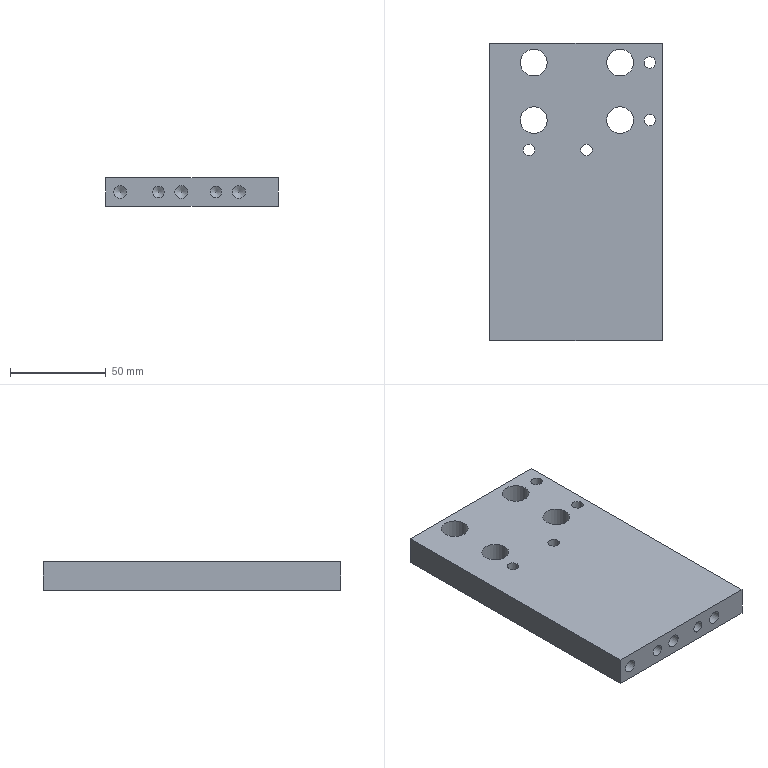Part | NX | features BREP 1 | 1 solid | 24 faces | box 90 x 155 x 15 mm | volume 195379 mm3 | cylinder 13 | plane 6 | cone 5 | commonest cylinder face diameters 6 x6 14 x4 6.8 x3
STEP:
#1=CARTESIAN_POINT('',(45.,-77.5,-7.5));
#2=VERTEX_POINT('',#1);
#3=CARTESIAN_POINT('',(45.,77.5,-7.5));
#4=VERTEX_POINT('',#3);
#5=CARTESIAN_POINT('',(45.,-77.5,-7.5));
#6=DIRECTION('',(0.,1.,0.));
#7=VECTOR('',#6,1000.);
#8=LINE('',#5,#7);
#9=EDGE_CURVE('',#2,#4,#8,.T.);
#10=ORIENTED_EDGE('',*,*,#9,.T.);
#11=CARTESIAN_POINT('',(45.,77.5,7.5));
#12=VERTEX_POINT('',#11);
#13=CARTESIAN_POINT('',(45.,77.5,7.5));
#14=DIRECTION('',(0.,0.,-1.));
#15=VECTOR('',#14,1000.);
#16=LINE('',#13,#15);
#17=EDGE_CURVE('',#12,#4,#16,.T.);
#18=ORIENTED_EDGE('',*,*,#17,.F.);
#19=CARTESIAN_POINT('',(45.,-77.5,7.5));
#20=VERTEX_POINT('',#19);
#21=CARTESIAN_POINT('',(45.,-77.5,7.5));
#22=DIRECTION('',(0.,1.,0.));
#23=VECTOR('',#22,1000.);
#24=LINE('',#21,#23);
#25=EDGE_CURVE('',#20,#12,#24,.T.);
#26=ORIENTED_EDGE('',*,*,#25,.F.);
#27=CARTESIAN_POINT('',(45.,-77.5,7.5));
#28=DIRECTION('',(0.,0.,-1.));
#29=VECTOR('',#28,1000.);
#30=LINE('',#27,#29);
#31=EDGE_CURVE('',#20,#2,#30,.T.);
#32=ORIENTED_EDGE('',*,*,#31,.T.);
#33=EDGE_LOOP('',(#10,#18,#26,#32));
#34=FACE_BOUND('',#33,.T.);
#35=CARTESIAN_POINT('',(45.,-77.5,7.5));
#36=DIRECTION('',(-1.,0.,0.));
#37=DIRECTION('',(0.,0.,-1.));
#38=AXIS2_PLACEMENT_3D('',#35,#36,#37);
#39=PLANE('',#38);
#40=ADVANCED_FACE('',(#34),#39,.F.);
#41=CARTESIAN_POINT('',(-45.,77.5,-7.5));
#42=VERTEX_POINT('',#41);
#43=CARTESIAN_POINT('',(-45.,77.5,-7.5));
#44=DIRECTION('',(-1.,0.,0.));
#45=VECTOR('',#44,1000.);
#46=LINE('',#43,#45);
#47=EDGE_CURVE('',#4,#42,#46,.T.);
#48=ORIENTED_EDGE('',*,*,#47,.T.);
#49=CARTESIAN_POINT('',(-45.,77.5,7.5));
#50=VERTEX_POINT('',#49);
#51=CARTESIAN_POINT('',(-45.,77.5,7.5));
#52=DIRECTION('',(0.,0.,-1.));
#53=VECTOR('',#52,1000.);
#54=LINE('',#51,#53);
#55=EDGE_CURVE('',#50,#42,#54,.T.);
#56=ORIENTED_EDGE('',*,*,#55,.F.);
#57=CARTESIAN_POINT('',(-45.,77.5,7.5));
#58=DIRECTION('',(-1.,0.,0.));
#59=VECTOR('',#58,1000.);
#60=LINE('',#57,#59);
#61=EDGE_CURVE('',#12,#50,#60,.T.);
#62=ORIENTED_EDGE('',*,*,#61,.F.);
#63=ORIENTED_EDGE('',*,*,#17,.T.);
#64=EDGE_LOOP('',(#48,#56,#62,#63));
#65=FACE_BOUND('',#64,.T.);
#66=CARTESIAN_POINT('',(-45.,77.5,7.5));
#67=DIRECTION('',(0.,-1.,0.));
#68=DIRECTION('',(0.,0.,1.));
#69=AXIS2_PLACEMENT_3D('',#66,#67,#68);
#70=PLANE('',#69);
#71=ADVANCED_FACE('',(#65),#70,.F.);
#72=CARTESIAN_POINT('',(-45.,-77.5,-7.5));
#73=VERTEX_POINT('',#72);
#74=CARTESIAN_POINT('',(-45.,-77.5,-7.5));
#75=DIRECTION('',(0.,-1.,0.));
#76=VECTOR('',#75,1000.);
#77=LINE('',#74,#76);
#78=EDGE_CURVE('',#42,#73,#77,.T.);
#79=ORIENTED_EDGE('',*,*,#78,.T.);
#80=CARTESIAN_POINT('',(-45.,-77.5,7.5));
#81=VERTEX_POINT('',#80);
#82=CARTESIAN_POINT('',(-45.,-77.5,7.5));
#83=DIRECTION('',(0.,0.,-1.));
#84=VECTOR('',#83,1000.);
#85=LINE('',#82,#84);
#86=EDGE_CURVE('',#81,#73,#85,.T.);
#87=ORIENTED_EDGE('',*,*,#86,.F.);
#88=CARTESIAN_POINT('',(-45.,-77.5,7.5));
#89=DIRECTION('',(0.,-1.,0.));
#90=VECTOR('',#89,1000.);
#91=LINE('',#88,#90);
#92=EDGE_CURVE('',#50,#81,#91,.T.);
#93=ORIENTED_EDGE('',*,*,#92,.F.);
#94=ORIENTED_EDGE('',*,*,#55,.T.);
#95=EDGE_LOOP('',(#79,#87,#93,#94));
#96=FACE_BOUND('',#95,.T.);
#97=CARTESIAN_POINT('',(-45.,-77.5,7.5));
#98=DIRECTION('',(1.,0.,0.));
#99=DIRECTION('',(0.,0.,1.));
#100=AXIS2_PLACEMENT_3D('',#97,#98,#99);
#101=PLANE('',#100);
#102=ADVANCED_FACE('',(#96),#101,.F.);
#103=CARTESIAN_POINT('',(-5.5,-77.5,-3.4));
#104=VERTEX_POINT('',#103);
#105=CARTESIAN_POINT('',(-5.5,-77.5,0.));
#106=DIRECTION('',(0.,-1.,0.));
#107=DIRECTION('',(0.,0.,-1.));
#108=AXIS2_PLACEMENT_3D('',#105,#106,#107);
#109=CIRCLE('',#108,3.4);
#110=EDGE_CURVE('',#104,#104,#109,.T.);
#111=ORIENTED_EDGE('',*,*,#110,.F.);
#112=EDGE_LOOP('',(#111));
#113=FACE_BOUND('',#112,.T.);
#114=CARTESIAN_POINT('',(24.5,-77.5,-3.4));
#115=VERTEX_POINT('',#114);
#116=CARTESIAN_POINT('',(24.5,-77.5,0.));
#117=DIRECTION('',(0.,-1.,0.));
#118=DIRECTION('',(0.,0.,-1.));
#119=AXIS2_PLACEMENT_3D('',#116,#117,#118);
#120=CIRCLE('',#119,3.4);
#121=EDGE_CURVE('',#115,#115,#120,.T.);
#122=ORIENTED_EDGE('',*,*,#121,.F.);
#123=EDGE_LOOP('',(#122));
#124=FACE_BOUND('',#123,.T.);
#125=CARTESIAN_POINT('',(-37.5,-77.5,-3.4));
#126=VERTEX_POINT('',#125);
#127=CARTESIAN_POINT('',(-37.5,-77.5,0.));
#128=DIRECTION('',(0.,-1.,0.));
#129=DIRECTION('',(0.,0.,-1.));
#130=AXIS2_PLACEMENT_3D('',#127,#128,#129);
#131=CIRCLE('',#130,3.4);
#132=EDGE_CURVE('',#126,#126,#131,.T.);
#133=ORIENTED_EDGE('',*,*,#132,.F.);
#134=EDGE_LOOP('',(#133));
#135=FACE_BOUND('',#134,.T.);
#136=CARTESIAN_POINT('',(-17.5,-77.5,-3.));
#137=VERTEX_POINT('',#136);
#138=CARTESIAN_POINT('',(-17.5,-77.5,0.));
#139=DIRECTION('',(0.,-1.,0.));
#140=DIRECTION('',(0.,0.,-1.));
#141=AXIS2_PLACEMENT_3D('',#138,#139,#140);
#142=CIRCLE('',#141,3.);
#143=EDGE_CURVE('',#137,#137,#142,.T.);
#144=ORIENTED_EDGE('',*,*,#143,.F.);
#145=EDGE_LOOP('',(#144));
#146=FACE_BOUND('',#145,.T.);
#147=CARTESIAN_POINT('',(12.5,-77.5,-3.));
#148=VERTEX_POINT('',#147);
#149=CARTESIAN_POINT('',(12.5,-77.5,0.));
#150=DIRECTION('',(0.,-1.,0.));
#151=DIRECTION('',(0.,0.,-1.));
#152=AXIS2_PLACEMENT_3D('',#149,#150,#151);
#153=CIRCLE('',#152,3.);
#154=EDGE_CURVE('',#148,#148,#153,.T.);
#155=ORIENTED_EDGE('',*,*,#154,.F.);
#156=EDGE_LOOP('',(#155));
#157=FACE_BOUND('',#156,.T.);
#158=CARTESIAN_POINT('',(-45.,-77.5,-7.5));
#159=DIRECTION('',(1.,0.,0.));
#160=VECTOR('',#159,1000.);
#161=LINE('',#158,#160);
#162=EDGE_CURVE('',#73,#2,#161,.T.);
#163=ORIENTED_EDGE('',*,*,#162,.T.);
#164=ORIENTED_EDGE('',*,*,#31,.F.);
#165=CARTESIAN_POINT('',(-45.,-77.5,7.5));
#166=DIRECTION('',(1.,0.,0.));
#167=VECTOR('',#166,1000.);
#168=LINE('',#165,#167);
#169=EDGE_CURVE('',#81,#20,#168,.T.);
#170=ORIENTED_EDGE('',*,*,#169,.F.);
#171=ORIENTED_EDGE('',*,*,#86,.T.);
#172=EDGE_LOOP('',(#163,#164,#170,#171));
#173=FACE_BOUND('',#172,.T.);
#174=CARTESIAN_POINT('',(-45.,-77.5,7.5));
#175=DIRECTION('',(0.,1.,0.));
#176=DIRECTION('',(0.,0.,-1.));
#177=AXIS2_PLACEMENT_3D('',#174,#175,#176);
#178=PLANE('',#177);
#179=ADVANCED_FACE('',(#113,#124,#135,#146,#157,#173),#178,.F.);
#180=CARTESIAN_POINT('',(30.,67.5,7.5));
#181=VERTEX_POINT('',#180);
#182=CARTESIAN_POINT('',(23.,67.5,7.5));
#183=DIRECTION('',(0.,0.,1.));
#184=DIRECTION('',(1.,0.,0.));
#185=AXIS2_PLACEMENT_3D('',#182,#183,#184);
#186=CIRCLE('',#185,7.);
#187=EDGE_CURVE('',#181,#181,#186,.T.);
#188=ORIENTED_EDGE('',*,*,#187,.F.);
#189=EDGE_LOOP('',(#188));
#190=FACE_BOUND('',#189,.T.);
#191=CARTESIAN_POINT('',(30.,37.5,7.5));
#192=VERTEX_POINT('',#191);
#193=CARTESIAN_POINT('',(23.,37.5,7.5));
#194=DIRECTION('',(0.,0.,1.));
#195=DIRECTION('',(1.,0.,0.));
#196=AXIS2_PLACEMENT_3D('',#193,#194,#195);
#197=CIRCLE('',#196,7.);
#198=EDGE_CURVE('',#192,#192,#197,.T.);
#199=ORIENTED_EDGE('',*,*,#198,.F.);
#200=EDGE_LOOP('',(#199));
#201=FACE_BOUND('',#200,.T.);
#202=CARTESIAN_POINT('',(-15.,37.5,7.5));
#203=VERTEX_POINT('',#202);
#204=CARTESIAN_POINT('',(-22.,37.5,7.5));
#205=DIRECTION('',(0.,0.,1.));
#206=DIRECTION('',(1.,0.,0.));
#207=AXIS2_PLACEMENT_3D('',#204,#205,#206);
#208=CIRCLE('',#207,7.);
#209=EDGE_CURVE('',#203,#203,#208,.T.);
#210=ORIENTED_EDGE('',*,*,#209,.F.);
#211=EDGE_LOOP('',(#210));
#212=FACE_BOUND('',#211,.T.);
#213=CARTESIAN_POINT('',(-15.,67.5,7.5));
#214=VERTEX_POINT('',#213);
#215=CARTESIAN_POINT('',(-22.,67.5,7.5));
#216=DIRECTION('',(0.,0.,1.));
#217=DIRECTION('',(1.,0.,0.));
#218=AXIS2_PLACEMENT_3D('',#215,#216,#217);
#219=CIRCLE('',#218,7.);
#220=EDGE_CURVE('',#214,#214,#219,.T.);
#221=ORIENTED_EDGE('',*,*,#220,.F.);
#222=EDGE_LOOP('',(#221));
#223=FACE_BOUND('',#222,.T.);
#224=CARTESIAN_POINT('',(35.5,67.5,7.5));
#225=VERTEX_POINT('',#224);
#226=CARTESIAN_POINT('',(38.5,67.5,7.5));
#227=DIRECTION('',(0.,0.,-1.));
#228=DIRECTION('',(-1.,0.,0.));
#229=AXIS2_PLACEMENT_3D('',#226,#227,#228);
#230=CIRCLE('',#229,3.);
#231=EDGE_CURVE('',#225,#225,#230,.T.);
#232=ORIENTED_EDGE('',*,*,#231,.T.);
#233=EDGE_LOOP('',(#232));
#234=FACE_BOUND('',#233,.T.);
#235=CARTESIAN_POINT('',(35.5,37.5,7.5));
#236=VERTEX_POINT('',#235);
#237=CARTESIAN_POINT('',(38.5,37.5,7.5));
#238=DIRECTION('',(0.,0.,-1.));
#239=DIRECTION('',(-1.,0.,0.));
#240=AXIS2_PLACEMENT_3D('',#237,#238,#239);
#241=CIRCLE('',#240,3.);
#242=EDGE_CURVE('',#236,#236,#241,.T.);
#243=ORIENTED_EDGE('',*,*,#242,.T.);
#244=EDGE_LOOP('',(#243));
#245=FACE_BOUND('',#244,.T.);
#246=CARTESIAN_POINT('',(2.5,22.,7.5));
#247=VERTEX_POINT('',#246);
#248=CARTESIAN_POINT('',(5.5,22.,7.5));
#249=DIRECTION('',(0.,0.,-1.));
#250=DIRECTION('',(-1.,0.,0.));
#251=AXIS2_PLACEMENT_3D('',#248,#249,#250);
#252=CIRCLE('',#251,3.);
#253=EDGE_CURVE('',#247,#247,#252,.T.);
#254=ORIENTED_EDGE('',*,*,#253,.T.);
#255=EDGE_LOOP('',(#254));
#256=FACE_BOUND('',#255,.T.);
#257=CARTESIAN_POINT('',(-27.5,22.,7.5));
#258=VERTEX_POINT('',#257);
#259=CARTESIAN_POINT('',(-24.5,22.,7.5));
#260=DIRECTION('',(0.,0.,-1.));
#261=DIRECTION('',(-1.,0.,0.));
#262=AXIS2_PLACEMENT_3D('',#259,#260,#261);
#263=CIRCLE('',#262,3.);
#264=EDGE_CURVE('',#258,#258,#263,.T.);
#265=ORIENTED_EDGE('',*,*,#264,.T.);
#266=EDGE_LOOP('',(#265));
#267=FACE_BOUND('',#266,.T.);
#268=ORIENTED_EDGE('',*,*,#25,.T.);
#269=ORIENTED_EDGE('',*,*,#61,.T.);
#270=ORIENTED_EDGE('',*,*,#92,.T.);
#271=ORIENTED_EDGE('',*,*,#169,.T.);
#272=EDGE_LOOP('',(#268,#269,#270,#271));
#273=FACE_BOUND('',#272,.T.);
#274=CARTESIAN_POINT('',(0.,0.,7.5));
#275=DIRECTION('',(0.,0.,-1.));
#276=DIRECTION('',(1.,0.,0.));
#277=AXIS2_PLACEMENT_3D('',#274,#275,#276);
#278=PLANE('',#277);
#279=ADVANCED_FACE('',(#190,#201,#212,#223,#234,#245,#256,#267,#273),#278,.F.);
#280=CARTESIAN_POINT('',(30.,67.5,-7.5));
#281=VERTEX_POINT('',#280);
#282=CARTESIAN_POINT('',(23.,67.5,-7.5));
#283=DIRECTION('',(0.,0.,1.));
#284=DIRECTION('',(1.,0.,0.));
#285=AXIS2_PLACEMENT_3D('',#282,#283,#284);
#286=CIRCLE('',#285,7.);
#287=EDGE_CURVE('',#281,#281,#286,.T.);
#288=ORIENTED_EDGE('',*,*,#287,.T.);
#289=EDGE_LOOP('',(#288));
#290=FACE_BOUND('',#289,.T.);
#291=CARTESIAN_POINT('',(30.,37.5,-7.5));
#292=VERTEX_POINT('',#291);
#293=CARTESIAN_POINT('',(23.,37.5,-7.5));
#294=DIRECTION('',(0.,0.,1.));
#295=DIRECTION('',(1.,0.,0.));
#296=AXIS2_PLACEMENT_3D('',#293,#294,#295);
#297=CIRCLE('',#296,7.);
#298=EDGE_CURVE('',#292,#292,#297,.T.);
#299=ORIENTED_EDGE('',*,*,#298,.T.);
#300=EDGE_LOOP('',(#299));
#301=FACE_BOUND('',#300,.T.);
#302=CARTESIAN_POINT('',(-15.,37.5,-7.5));
#303=VERTEX_POINT('',#302);
#304=CARTESIAN_POINT('',(-22.,37.5,-7.5));
#305=DIRECTION('',(0.,0.,1.));
#306=DIRECTION('',(1.,0.,0.));
#307=AXIS2_PLACEMENT_3D('',#304,#305,#306);
#308=CIRCLE('',#307,7.);
#309=EDGE_CURVE('',#303,#303,#308,.T.);
#310=ORIENTED_EDGE('',*,*,#309,.T.);
#311=EDGE_LOOP('',(#310));
#312=FACE_BOUND('',#311,.T.);
#313=CARTESIAN_POINT('',(-15.,67.5,-7.5));
#314=VERTEX_POINT('',#313);
#315=CARTESIAN_POINT('',(-22.,67.5,-7.5));
#316=DIRECTION('',(0.,0.,1.));
#317=DIRECTION('',(1.,0.,0.));
#318=AXIS2_PLACEMENT_3D('',#315,#316,#317);
#319=CIRCLE('',#318,7.);
#320=EDGE_CURVE('',#314,#314,#319,.T.);
#321=ORIENTED_EDGE('',*,*,#320,.T.);
#322=EDGE_LOOP('',(#321));
#323=FACE_BOUND('',#322,.T.);
#324=CARTESIAN_POINT('',(35.5,67.5,-7.5));
#325=VERTEX_POINT('',#324);
#326=CARTESIAN_POINT('',(38.5,67.5,-7.5));
#327=DIRECTION('',(0.,0.,-1.));
#328=DIRECTION('',(-1.,0.,0.));
#329=AXIS2_PLACEMENT_3D('',#326,#327,#328);
#330=CIRCLE('',#329,3.);
#331=EDGE_CURVE('',#325,#325,#330,.T.);
#332=ORIENTED_EDGE('',*,*,#331,.F.);
#333=EDGE_LOOP('',(#332));
#334=FACE_BOUND('',#333,.T.);
#335=CARTESIAN_POINT('',(35.5,37.5,-7.5));
#336=VERTEX_POINT('',#335);
#337=CARTESIAN_POINT('',(38.5,37.5,-7.5));
#338=DIRECTION('',(0.,0.,-1.));
#339=DIRECTION('',(-1.,0.,0.));
#340=AXIS2_PLACEMENT_3D('',#337,#338,#339);
#341=CIRCLE('',#340,3.);
#342=EDGE_CURVE('',#336,#336,#341,.T.);
#343=ORIENTED_EDGE('',*,*,#342,.F.);
#344=EDGE_LOOP('',(#343));
#345=FACE_BOUND('',#344,.T.);
#346=CARTESIAN_POINT('',(2.5,22.,-7.5));
#347=VERTEX_POINT('',#346);
#348=CARTESIAN_POINT('',(5.5,22.,-7.5));
#349=DIRECTION('',(0.,0.,-1.));
#350=DIRECTION('',(-1.,0.,0.));
#351=AXIS2_PLACEMENT_3D('',#348,#349,#350);
#352=CIRCLE('',#351,3.);
#353=EDGE_CURVE('',#347,#347,#352,.T.);
#354=ORIENTED_EDGE('',*,*,#353,.F.);
#355=EDGE_LOOP('',(#354));
#356=FACE_BOUND('',#355,.T.);
#357=CARTESIAN_POINT('',(-27.5,22.,-7.5));
#358=VERTEX_POINT('',#357);
#359=CARTESIAN_POINT('',(-24.5,22.,-7.5));
#360=DIRECTION('',(0.,0.,-1.));
#361=DIRECTION('',(-1.,0.,0.));
#362=AXIS2_PLACEMENT_3D('',#359,#360,#361);
#363=CIRCLE('',#362,3.);
#364=EDGE_CURVE('',#358,#358,#363,.T.);
#365=ORIENTED_EDGE('',*,*,#364,.F.);
#366=EDGE_LOOP('',(#365));
#367=FACE_BOUND('',#366,.T.);
#368=ORIENTED_EDGE('',*,*,#9,.F.);
#369=ORIENTED_EDGE('',*,*,#162,.F.);
#370=ORIENTED_EDGE('',*,*,#78,.F.);
#371=ORIENTED_EDGE('',*,*,#47,.F.);
#372=EDGE_LOOP('',(#368,#369,#370,#371));
#373=FACE_BOUND('',#372,.T.);
#374=CARTESIAN_POINT('',(0.,0.,-7.5));
#375=DIRECTION('',(0.,0.,-1.));
#376=DIRECTION('',(1.,0.,0.));
#377=AXIS2_PLACEMENT_3D('',#374,#375,#376);
#378=PLANE('',#377);
#379=ADVANCED_FACE('',(#290,#301,#312,#323,#334,#345,#356,#367,#373),#378,.T.);
#380=ORIENTED_EDGE('',*,*,#264,.F.);
#381=EDGE_LOOP('',(#380));
#382=FACE_BOUND('',#381,.T.);
#383=ORIENTED_EDGE('',*,*,#364,.T.);
#384=EDGE_LOOP('',(#383));
#385=FACE_BOUND('',#384,.T.);
#386=CARTESIAN_POINT('',(-24.5,22.,-7.5));
#387=DIRECTION('',(0.,0.,-1.));
#388=DIRECTION('',(1.,0.,0.));
#389=AXIS2_PLACEMENT_3D('',#386,#387,#388);
#390=CYLINDRICAL_SURFACE('',#389,3.);
#391=ADVANCED_FACE('',(#382,#385),#390,.F.);
#392=ORIENTED_EDGE('',*,*,#253,.F.);
#393=EDGE_LOOP('',(#392));
#394=FACE_BOUND('',#393,.T.);
#395=ORIENTED_EDGE('',*,*,#353,.T.);
#396=EDGE_LOOP('',(#395));
#397=FACE_BOUND('',#396,.T.);
#398=CARTESIAN_POINT('',(5.5,22.,-7.5));
#399=DIRECTION('',(0.,0.,-1.));
#400=DIRECTION('',(1.,0.,0.));
#401=AXIS2_PLACEMENT_3D('',#398,#399,#400);
#402=CYLINDRICAL_SURFACE('',#401,3.);
#403=ADVANCED_FACE('',(#394,#397),#402,.F.);
#404=ORIENTED_EDGE('',*,*,#242,.F.);
#405=EDGE_LOOP('',(#404));
#406=FACE_BOUND('',#405,.T.);
#407=ORIENTED_EDGE('',*,*,#342,.T.);
#408=EDGE_LOOP('',(#407));
#409=FACE_BOUND('',#408,.T.);
#410=CARTESIAN_POINT('',(38.5,37.5,-7.5));
#411=DIRECTION('',(0.,0.,-1.));
#412=DIRECTION('',(1.,0.,0.));
#413=AXIS2_PLACEMENT_3D('',#410,#411,#412);
#414=CYLINDRICAL_SURFACE('',#413,3.);
#415=ADVANCED_FACE('',(#406,#409),#414,.F.);
#416=ORIENTED_EDGE('',*,*,#231,.F.);
#417=EDGE_LOOP('',(#416));
#418=FACE_BOUND('',#417,.T.);
#419=ORIENTED_EDGE('',*,*,#331,.T.);
#420=EDGE_LOOP('',(#419));
#421=FACE_BOUND('',#420,.T.);
#422=CARTESIAN_POINT('',(38.5,67.5,-7.5));
#423=DIRECTION('',(0.,0.,-1.));
#424=DIRECTION('',(1.,0.,0.));
#425=AXIS2_PLACEMENT_3D('',#422,#423,#424);
#426=CYLINDRICAL_SURFACE('',#425,3.);
#427=ADVANCED_FACE('',(#418,#421),#426,.F.);
#428=ORIENTED_EDGE('',*,*,#320,.F.);
#429=EDGE_LOOP('',(#428));
#430=FACE_BOUND('',#429,.T.);
#431=ORIENTED_EDGE('',*,*,#220,.T.);
#432=EDGE_LOOP('',(#431));
#433=FACE_BOUND('',#432,.T.);
#434=CARTESIAN_POINT('',(-22.,67.5,7.5));
#435=DIRECTION('',(0.,0.,1.));
#436=DIRECTION('',(-1.,0.,0.));
#437=AXIS2_PLACEMENT_3D('',#434,#435,#436);
#438=CYLINDRICAL_SURFACE('',#437,7.);
#439=ADVANCED_FACE('',(#430,#433),#438,.F.);
#440=ORIENTED_EDGE('',*,*,#309,.F.);
#441=EDGE_LOOP('',(#440));
#442=FACE_BOUND('',#441,.T.);
#443=ORIENTED_EDGE('',*,*,#209,.T.);
#444=EDGE_LOOP('',(#443));
#445=FACE_BOUND('',#444,.T.);
#446=CARTESIAN_POINT('',(-22.,37.5,7.5));
#447=DIRECTION('',(0.,0.,1.));
#448=DIRECTION('',(-1.,0.,0.));
#449=AXIS2_PLACEMENT_3D('',#446,#447,#448);
#450=CYLINDRICAL_SURFACE('',#449,7.);
#451=ADVANCED_FACE('',(#442,#445),#450,.F.);
#452=ORIENTED_EDGE('',*,*,#298,.F.);
#453=EDGE_LOOP('',(#452));
#454=FACE_BOUND('',#453,.T.);
#455=ORIENTED_EDGE('',*,*,#198,.T.);
#456=EDGE_LOOP('',(#455));
#457=FACE_BOUND('',#456,.T.);
#458=CARTESIAN_POINT('',(23.,37.5,7.5));
#459=DIRECTION('',(0.,0.,1.));
#460=DIRECTION('',(-1.,0.,0.));
#461=AXIS2_PLACEMENT_3D('',#458,#459,#460);
#462=CYLINDRICAL_SURFACE('',#461,7.);
#463=ADVANCED_FACE('',(#454,#457),#462,.F.);
#464=ORIENTED_EDGE('',*,*,#287,.F.);
#465=EDGE_LOOP('',(#464));
#466=FACE_BOUND('',#465,.T.);
#467=ORIENTED_EDGE('',*,*,#187,.T.);
#468=EDGE_LOOP('',(#467));
#469=FACE_BOUND('',#468,.T.);
#470=CARTESIAN_POINT('',(23.,67.5,7.5));
#471=DIRECTION('',(0.,0.,1.));
#472=DIRECTION('',(-1.,0.,0.));
#473=AXIS2_PLACEMENT_3D('',#470,#471,#472);
#474=CYLINDRICAL_SURFACE('',#473,7.);
#475=ADVANCED_FACE('',(#466,#469),#474,.F.);
#476=CARTESIAN_POINT('',(12.5,-63.697,0.));
#477=VERTEX_POINT('',#476);
#478=VERTEX_LOOP('',#477);
#479=FACE_BOUND('',#478,.T.);
#480=CARTESIAN_POINT('',(12.5,-65.5,-3.));
#481=VERTEX_POINT('',#480);
#482=CARTESIAN_POINT('',(12.5,-65.5,0.));
#483=DIRECTION('',(0.,-1.,0.));
#484=DIRECTION('',(0.,0.,-1.));
#485=AXIS2_PLACEMENT_3D('',#482,#483,#484);
#486=CIRCLE('',#485,3.);
#487=EDGE_CURVE('',#481,#481,#486,.T.);
#488=ORIENTED_EDGE('',*,*,#487,.T.);
#489=EDGE_LOOP('',(#488));
#490=FACE_BOUND('',#489,.T.);
#491=CARTESIAN_POINT('',(12.5,-65.5,0.));
#492=DIRECTION('',(0.,-1.,0.));
#493=DIRECTION('',(0.,0.,1.));
#494=AXIS2_PLACEMENT_3D('',#491,#492,#493);
#495=CONICAL_SURFACE('',#494,3.,1.03);
#496=ADVANCED_FACE('',(#479,#490),#495,.F.);
#497=ORIENTED_EDGE('',*,*,#487,.F.);
#498=EDGE_LOOP('',(#497));
#499=FACE_BOUND('',#498,.T.);
#500=ORIENTED_EDGE('',*,*,#154,.T.);
#501=EDGE_LOOP('',(#500));
#502=FACE_BOUND('',#501,.T.);
#503=CARTESIAN_POINT('',(12.5,-77.5,0.));
#504=DIRECTION('',(0.,-1.,0.));
#505=DIRECTION('',(0.,0.,1.));
#506=AXIS2_PLACEMENT_3D('',#503,#504,#505);
#507=CYLINDRICAL_SURFACE('',#506,3.);
#508=ADVANCED_FACE('',(#499,#502),#507,.F.);
#509=CARTESIAN_POINT('',(-17.5,-63.697,0.));
#510=VERTEX_POINT('',#509);
#511=VERTEX_LOOP('',#510);
#512=FACE_BOUND('',#511,.T.);
#513=CARTESIAN_POINT('',(-17.5,-65.5,-3.));
#514=VERTEX_POINT('',#513);
#515=CARTESIAN_POINT('',(-17.5,-65.5,0.));
#516=DIRECTION('',(0.,-1.,0.));
#517=DIRECTION('',(0.,0.,-1.));
#518=AXIS2_PLACEMENT_3D('',#515,#516,#517);
#519=CIRCLE('',#518,3.);
#520=EDGE_CURVE('',#514,#514,#519,.T.);
#521=ORIENTED_EDGE('',*,*,#520,.T.);
#522=EDGE_LOOP('',(#521));
#523=FACE_BOUND('',#522,.T.);
#524=CARTESIAN_POINT('',(-17.5,-65.5,0.));
#525=DIRECTION('',(0.,-1.,0.));
#526=DIRECTION('',(0.,0.,1.));
#527=AXIS2_PLACEMENT_3D('',#524,#525,#526);
#528=CONICAL_SURFACE('',#527,3.,1.03);
#529=ADVANCED_FACE('',(#512,#523),#528,.F.);
#530=ORIENTED_EDGE('',*,*,#520,.F.);
#531=EDGE_LOOP('',(#530));
#532=FACE_BOUND('',#531,.T.);
#533=ORIENTED_EDGE('',*,*,#143,.T.);
#534=EDGE_LOOP('',(#533));
#535=FACE_BOUND('',#534,.T.);
#536=CARTESIAN_POINT('',(-17.5,-77.5,0.));
#537=DIRECTION('',(0.,-1.,0.));
#538=DIRECTION('',(0.,0.,1.));
#539=AXIS2_PLACEMENT_3D('',#536,#537,#538);
#540=CYLINDRICAL_SURFACE('',#539,3.);
#541=ADVANCED_FACE('',(#532,#535),#540,.F.);
#542=CARTESIAN_POINT('',(-37.5,-55.707,0.));
#543=VERTEX_POINT('',#542);
#544=VERTEX_LOOP('',#543);
#545=FACE_BOUND('',#544,.T.);
#546=CARTESIAN_POINT('',(-37.5,-57.75,-3.4));
#547=VERTEX_POINT('',#546);
#548=CARTESIAN_POINT('',(-37.5,-57.75,0.));
#549=DIRECTION('',(0.,-1.,0.));
#550=DIRECTION('',(0.,0.,-1.));
#551=AXIS2_PLACEMENT_3D('',#548,#549,#550);
#552=CIRCLE('',#551,3.4);
#553=EDGE_CURVE('',#547,#547,#552,.T.);
#554=ORIENTED_EDGE('',*,*,#553,.T.);
#555=EDGE_LOOP('',(#554));
#556=FACE_BOUND('',#555,.T.);
#557=CARTESIAN_POINT('',(-37.5,-57.75,0.));
#558=DIRECTION('',(0.,-1.,0.));
#559=DIRECTION('',(0.,0.,1.));
#560=AXIS2_PLACEMENT_3D('',#557,#558,#559);
#561=CONICAL_SURFACE('',#560,3.4,1.03);
#562=ADVANCED_FACE('',(#545,#556),#561,.F.);
#563=ORIENTED_EDGE('',*,*,#553,.F.);
#564=EDGE_LOOP('',(#563));
#565=FACE_BOUND('',#564,.T.);
#566=ORIENTED_EDGE('',*,*,#132,.T.);
#567=EDGE_LOOP('',(#566));
#568=FACE_BOUND('',#567,.T.);
#569=CARTESIAN_POINT('',(-37.5,-77.5,0.));
#570=DIRECTION('',(0.,-1.,0.));
#571=DIRECTION('',(0.,0.,1.));
#572=AXIS2_PLACEMENT_3D('',#569,#570,#571);
#573=CYLINDRICAL_SURFACE('',#572,3.4);
#574=ADVANCED_FACE('',(#565,#568),#573,.F.);
#575=CARTESIAN_POINT('',(24.5,-55.707,0.));
#576=VERTEX_POINT('',#575);
#577=VERTEX_LOOP('',#576);
#578=FACE_BOUND('',#577,.T.);
#579=CARTESIAN_POINT('',(24.5,-57.75,-3.4));
#580=VERTEX_POINT('',#579);
#581=CARTESIAN_POINT('',(24.5,-57.75,0.));
#582=DIRECTION('',(0.,-1.,0.));
#583=DIRECTION('',(0.,0.,-1.));
#584=AXIS2_PLACEMENT_3D('',#581,#582,#583);
#585=CIRCLE('',#584,3.4);
#586=EDGE_CURVE('',#580,#580,#585,.T.);
#587=ORIENTED_EDGE('',*,*,#586,.T.);
#588=EDGE_LOOP('',(#587));
#589=FACE_BOUND('',#588,.T.);
#590=CARTESIAN_POINT('',(24.5,-57.75,0.));
#591=DIRECTION('',(0.,-1.,0.));
#592=DIRECTION('',(0.,0.,1.));
#593=AXIS2_PLACEMENT_3D('',#590,#591,#592);
#594=CONICAL_SURFACE('',#593,3.4,1.03);
#595=ADVANCED_FACE('',(#578,#589),#594,.F.);
#596=ORIENTED_EDGE('',*,*,#586,.F.);
#597=EDGE_LOOP('',(#596));
#598=FACE_BOUND('',#597,.T.);
#599=ORIENTED_EDGE('',*,*,#121,.T.);
#600=EDGE_LOOP('',(#599));
#601=FACE_BOUND('',#600,.T.);
#602=CARTESIAN_POINT('',(24.5,-77.5,0.));
#603=DIRECTION('',(0.,-1.,0.));
#604=DIRECTION('',(0.,0.,1.));
#605=AXIS2_PLACEMENT_3D('',#602,#603,#604);
#606=CYLINDRICAL_SURFACE('',#605,3.4);
#607=ADVANCED_FACE('',(#598,#601),#606,.F.);
#608=CARTESIAN_POINT('',(-5.5,-55.707,0.));
#609=VERTEX_POINT('',#608);
#610=VERTEX_LOOP('',#609);
#611=FACE_BOUND('',#610,.T.);
#612=CARTESIAN_POINT('',(-5.5,-57.75,-3.4));
#613=VERTEX_POINT('',#612);
#614=CARTESIAN_POINT('',(-5.5,-57.75,0.));
#615=DIRECTION('',(0.,-1.,0.));
#616=DIRECTION('',(0.,0.,-1.));
#617=AXIS2_PLACEMENT_3D('',#614,#615,#616);
#618=CIRCLE('',#617,3.4);
#619=EDGE_CURVE('',#613,#613,#618,.T.);
#620=ORIENTED_EDGE('',*,*,#619,.T.);
#621=EDGE_LOOP('',(#620));
#622=FACE_BOUND('',#621,.T.);
#623=CARTESIAN_POINT('',(-5.5,-57.75,0.));
#624=DIRECTION('',(0.,-1.,0.));
#625=DIRECTION('',(0.,0.,1.));
#626=AXIS2_PLACEMENT_3D('',#623,#624,#625);
#627=CONICAL_SURFACE('',#626,3.4,1.03);
#628=ADVANCED_FACE('',(#611,#622),#627,.F.);
#629=ORIENTED_EDGE('',*,*,#619,.F.);
#630=EDGE_LOOP('',(#629));
#631=FACE_BOUND('',#630,.T.);
#632=ORIENTED_EDGE('',*,*,#110,.T.);
#633=EDGE_LOOP('',(#632));
#634=FACE_BOUND('',#633,.T.);
#635=CARTESIAN_POINT('',(-5.5,-77.5,0.));
#636=DIRECTION('',(0.,-1.,0.));
#637=DIRECTION('',(0.,0.,1.));
#638=AXIS2_PLACEMENT_3D('',#635,#636,#637);
#639=CYLINDRICAL_SURFACE('',#638,3.4);
#640=ADVANCED_FACE('',(#631,#634),#639,.F.);
#641=CLOSED_SHELL('',(#40,#71,#102,#179,#279,#379,#391,#403,#415,#427,#439,#451,#463,#475,#496,#508,#529,#541,#562,#574,#595,#607,#628,#640));
#642=MANIFOLD_SOLID_BREP('',#641);
#643=(LENGTH_UNIT()NAMED_UNIT(*)SI_UNIT(.MILLI.,.METRE.));
#644=UNCERTAINTY_MEASURE_WITH_UNIT(LENGTH_MEASURE(0.00001),#643,'','');
#645=(NAMED_UNIT(*)PLANE_ANGLE_UNIT()SI_UNIT($,.RADIAN.));
#646=(NAMED_UNIT(*)SI_UNIT($,.STERADIAN.)SOLID_ANGLE_UNIT());
#647=(GEOMETRIC_REPRESENTATION_CONTEXT(3)GLOBAL_UNCERTAINTY_ASSIGNED_CONTEXT((#644))GLOBAL_UNIT_ASSIGNED_CONTEXT((#643,#645,#646))REPRESENTATION_CONTEXT('',''));
#648=ADVANCED_BREP_SHAPE_REPRESENTATION('',(#642),#647);